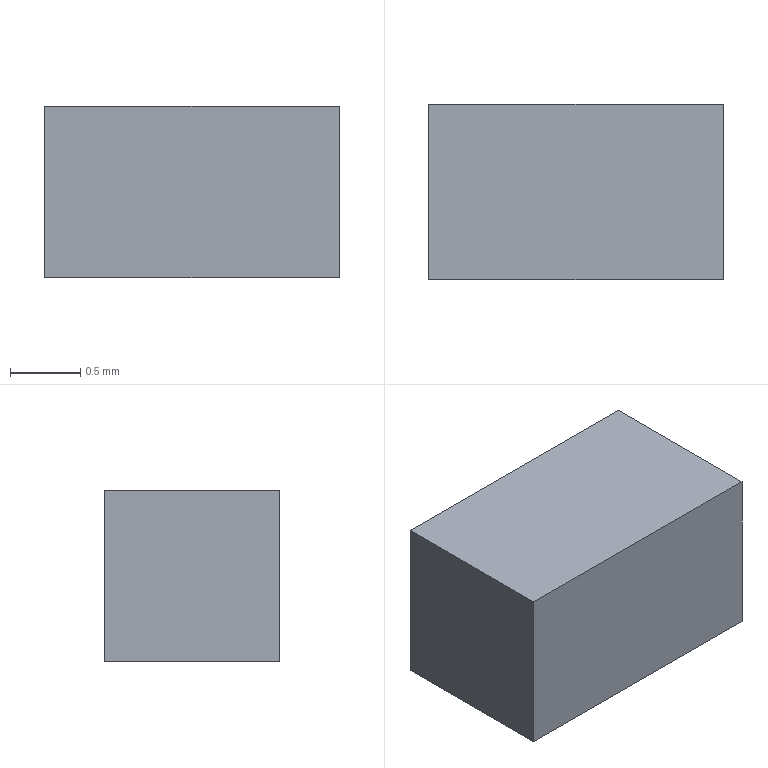Part | Creo | 1 solid | 6 faces | box 2.1 x 1.25 x 1.222 mm | volume 3.208 mm3 | plane 6
STEP:
#1=CARTESIAN_POINT('',(0.,0.,0.));
#2=DIRECTION('',(0.,0.,1.));
#3=DIRECTION('',(1.,0.,0.));
#4=AXIS2_PLACEMENT_3D('',#1,#2,#3);
#5=CARTESIAN_POINT('',(-1.05,-0.625,0.));
#6=VERTEX_POINT('',#5);
#7=CARTESIAN_POINT('',(1.05,-0.625,0.));
#8=VERTEX_POINT('',#7);
#9=CARTESIAN_POINT('',(-1.05,-0.625,0.));
#10=DIRECTION('',(1.,0.,0.));
#11=VECTOR('',#10,2.1);
#12=LINE('',#9,#11);
#13=EDGE_CURVE('',#6,#8,#12,.T.);
#14=ORIENTED_EDGE('',*,*,#13,.T.);
#15=CARTESIAN_POINT('',(1.05,0.625,0.));
#16=VERTEX_POINT('',#15);
#17=CARTESIAN_POINT('',(1.05,-0.625,0.));
#18=DIRECTION('',(0.,1.,0.));
#19=VECTOR('',#18,1.25);
#20=LINE('',#17,#19);
#21=EDGE_CURVE('',#8,#16,#20,.T.);
#22=ORIENTED_EDGE('',*,*,#21,.T.);
#23=CARTESIAN_POINT('',(-1.05,0.625,0.));
#24=VERTEX_POINT('',#23);
#25=CARTESIAN_POINT('',(1.05,0.625,0.));
#26=DIRECTION('',(-1.,0.,0.));
#27=VECTOR('',#26,2.1);
#28=LINE('',#25,#27);
#29=EDGE_CURVE('',#16,#24,#28,.T.);
#30=ORIENTED_EDGE('',*,*,#29,.T.);
#31=CARTESIAN_POINT('',(-1.05,0.625,0.));
#32=DIRECTION('',(0.,-1.,0.));
#33=VECTOR('',#32,1.25);
#34=LINE('',#31,#33);
#35=EDGE_CURVE('',#24,#6,#34,.T.);
#36=ORIENTED_EDGE('',*,*,#35,.T.);
#37=EDGE_LOOP('',(#14,#22,#30,#36));
#38=FACE_OUTER_BOUND('',#37,.F.);
#39=CARTESIAN_POINT('',(0.,0.,0.));
#40=DIRECTION('',(0.,0.,1.));
#41=DIRECTION('',(1.,0.,0.));
#42=AXIS2_PLACEMENT_3D('',#39,#40,#41);
#43=PLANE('',#42);
#44=ADVANCED_FACE('',(#38),#43,.F.);
#45=ORIENTED_EDGE('',*,*,#13,.F.);
#46=CARTESIAN_POINT('',(-1.05,-0.625,1.222));
#47=VERTEX_POINT('',#46);
#48=CARTESIAN_POINT('',(-1.05,-0.625,0.));
#49=DIRECTION('',(0.,0.,1.));
#50=VECTOR('',#49,1.222);
#51=LINE('',#48,#50);
#52=EDGE_CURVE('',#6,#47,#51,.T.);
#53=ORIENTED_EDGE('',*,*,#52,.T.);
#54=CARTESIAN_POINT('',(1.05,-0.625,1.222));
#55=VERTEX_POINT('',#54);
#56=CARTESIAN_POINT('',(-1.05,-0.625,1.222));
#57=DIRECTION('',(1.,0.,0.));
#58=VECTOR('',#57,2.1);
#59=LINE('',#56,#58);
#60=EDGE_CURVE('',#47,#55,#59,.T.);
#61=ORIENTED_EDGE('',*,*,#60,.T.);
#62=CARTESIAN_POINT('',(1.05,-0.625,0.));
#63=DIRECTION('',(0.,0.,1.));
#64=VECTOR('',#63,1.222);
#65=LINE('',#62,#64);
#66=EDGE_CURVE('',#8,#55,#65,.T.);
#67=ORIENTED_EDGE('',*,*,#66,.F.);
#68=EDGE_LOOP('',(#45,#53,#61,#67));
#69=FACE_OUTER_BOUND('',#68,.F.);
#70=CARTESIAN_POINT('',(-1.05,-0.625,0.));
#71=DIRECTION('',(0.,-1.,0.));
#72=DIRECTION('',(1.,0.,0.));
#73=AXIS2_PLACEMENT_3D('',#70,#71,#72);
#74=PLANE('',#73);
#75=ADVANCED_FACE('',(#69),#74,.T.);
#76=ORIENTED_EDGE('',*,*,#35,.F.);
#77=CARTESIAN_POINT('',(-1.05,0.625,1.222));
#78=VERTEX_POINT('',#77);
#79=CARTESIAN_POINT('',(-1.05,0.625,0.));
#80=DIRECTION('',(0.,0.,1.));
#81=VECTOR('',#80,1.222);
#82=LINE('',#79,#81);
#83=EDGE_CURVE('',#24,#78,#82,.T.);
#84=ORIENTED_EDGE('',*,*,#83,.T.);
#85=CARTESIAN_POINT('',(-1.05,0.625,1.222));
#86=DIRECTION('',(0.,-1.,0.));
#87=VECTOR('',#86,1.25);
#88=LINE('',#85,#87);
#89=EDGE_CURVE('',#78,#47,#88,.T.);
#90=ORIENTED_EDGE('',*,*,#89,.T.);
#91=ORIENTED_EDGE('',*,*,#52,.F.);
#92=EDGE_LOOP('',(#76,#84,#90,#91));
#93=FACE_OUTER_BOUND('',#92,.F.);
#94=CARTESIAN_POINT('',(-1.05,0.625,0.));
#95=DIRECTION('',(-1.,0.,0.));
#96=DIRECTION('',(0.,-1.,0.));
#97=AXIS2_PLACEMENT_3D('',#94,#95,#96);
#98=PLANE('',#97);
#99=ADVANCED_FACE('',(#93),#98,.T.);
#100=ORIENTED_EDGE('',*,*,#29,.F.);
#101=CARTESIAN_POINT('',(1.05,0.625,1.222));
#102=VERTEX_POINT('',#101);
#103=CARTESIAN_POINT('',(1.05,0.625,0.));
#104=DIRECTION('',(0.,0.,1.));
#105=VECTOR('',#104,1.222);
#106=LINE('',#103,#105);
#107=EDGE_CURVE('',#16,#102,#106,.T.);
#108=ORIENTED_EDGE('',*,*,#107,.T.);
#109=CARTESIAN_POINT('',(1.05,0.625,1.222));
#110=DIRECTION('',(-1.,0.,0.));
#111=VECTOR('',#110,2.1);
#112=LINE('',#109,#111);
#113=EDGE_CURVE('',#102,#78,#112,.T.);
#114=ORIENTED_EDGE('',*,*,#113,.T.);
#115=ORIENTED_EDGE('',*,*,#83,.F.);
#116=EDGE_LOOP('',(#100,#108,#114,#115));
#117=FACE_OUTER_BOUND('',#116,.F.);
#118=CARTESIAN_POINT('',(1.05,0.625,0.));
#119=DIRECTION('',(0.,1.,0.));
#120=DIRECTION('',(-1.,0.,0.));
#121=AXIS2_PLACEMENT_3D('',#118,#119,#120);
#122=PLANE('',#121);
#123=ADVANCED_FACE('',(#117),#122,.T.);
#124=ORIENTED_EDGE('',*,*,#21,.F.);
#125=ORIENTED_EDGE('',*,*,#66,.T.);
#126=CARTESIAN_POINT('',(1.05,-0.625,1.222));
#127=DIRECTION('',(0.,1.,0.));
#128=VECTOR('',#127,1.25);
#129=LINE('',#126,#128);
#130=EDGE_CURVE('',#55,#102,#129,.T.);
#131=ORIENTED_EDGE('',*,*,#130,.T.);
#132=ORIENTED_EDGE('',*,*,#107,.F.);
#133=EDGE_LOOP('',(#124,#125,#131,#132));
#134=FACE_OUTER_BOUND('',#133,.F.);
#135=CARTESIAN_POINT('',(1.05,-0.625,0.));
#136=DIRECTION('',(1.,0.,0.));
#137=DIRECTION('',(0.,1.,0.));
#138=AXIS2_PLACEMENT_3D('',#135,#136,#137);
#139=PLANE('',#138);
#140=ADVANCED_FACE('',(#134),#139,.T.);
#141=ORIENTED_EDGE('',*,*,#60,.F.);
#142=ORIENTED_EDGE('',*,*,#89,.F.);
#143=ORIENTED_EDGE('',*,*,#113,.F.);
#144=ORIENTED_EDGE('',*,*,#130,.F.);
#145=EDGE_LOOP('',(#141,#142,#143,#144));
#146=FACE_OUTER_BOUND('',#145,.F.);
#147=CARTESIAN_POINT('',(0.,0.,1.222));
#148=DIRECTION('',(0.,0.,1.));
#149=DIRECTION('',(1.,0.,0.));
#150=AXIS2_PLACEMENT_3D('',#147,#148,#149);
#151=PLANE('',#150);
#152=ADVANCED_FACE('',(#146),#151,.T.);
#153=CLOSED_SHELL('',(#44,#75,#99,#123,#140,#152));
#154=MANIFOLD_SOLID_BREP('',#153);
#155=(LENGTH_UNIT()NAMED_UNIT(*)SI_UNIT(.MILLI.,.METRE.));
#156=UNCERTAINTY_MEASURE_WITH_UNIT(LENGTH_MEASURE(0.0002732),#155,'','');
#157=(NAMED_UNIT(*)PLANE_ANGLE_UNIT()SI_UNIT($,.RADIAN.));
#158=PLANE_ANGLE_MEASURE_WITH_UNIT(PLANE_ANGLE_MEASURE(0.01745),#157);
#159=(CONVERSION_BASED_UNIT('DEGREE',#158)NAMED_UNIT(*)PLANE_ANGLE_UNIT());
#160=(NAMED_UNIT(*)SI_UNIT($,.STERADIAN.)SOLID_ANGLE_UNIT());
#161=(GEOMETRIC_REPRESENTATION_CONTEXT(3)GLOBAL_UNCERTAINTY_ASSIGNED_CONTEXT((#156))GLOBAL_UNIT_ASSIGNED_CONTEXT((#155,#159,#160))REPRESENTATION_CONTEXT('',''));
#162=ADVANCED_BREP_SHAPE_REPRESENTATION('',(#4,#154),#161);